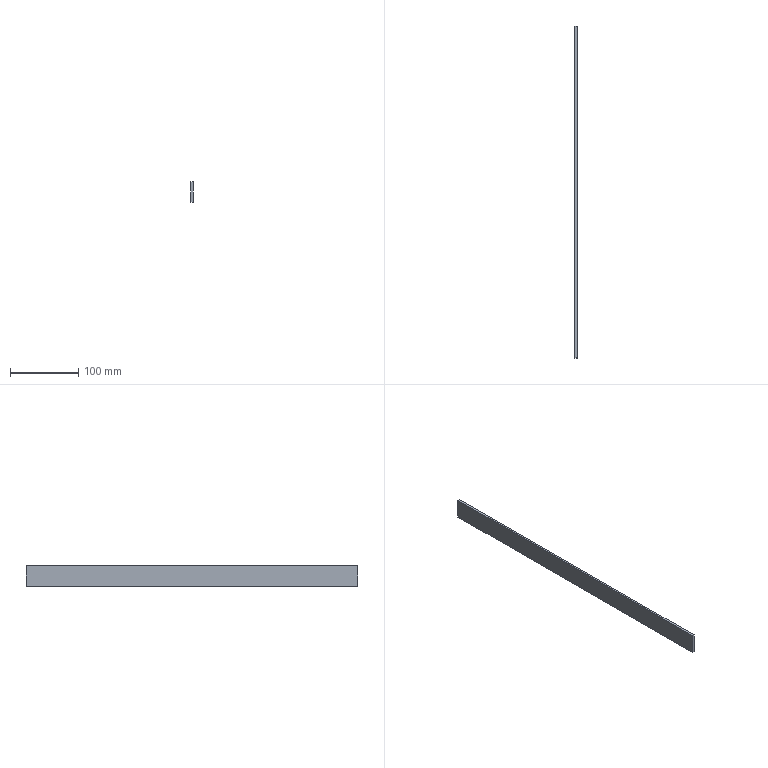Part | SolidWorks | 1 solid | 6 faces | box 3 x 485 x 30 mm | volume 43650 mm3 | plane 6
STEP:
#1=CARTESIAN_POINT('',(0.,242.5,15.));
#2=VERTEX_POINT('',#1);
#3=CARTESIAN_POINT('',(0.,-242.5,15.));
#4=VERTEX_POINT('',#3);
#5=CARTESIAN_POINT('',(0.,-242.5,15.));
#6=DIRECTION('',(0.,-1.,0.));
#7=VECTOR('',#6,1000.);
#8=LINE('',#5,#7);
#9=EDGE_CURVE('',#2,#4,#8,.T.);
#10=ORIENTED_EDGE('',*,*,#9,.F.);
#11=CARTESIAN_POINT('',(-3.,242.5,15.));
#12=VERTEX_POINT('',#11);
#13=CARTESIAN_POINT('',(-3.,242.5,15.));
#14=DIRECTION('',(1.,0.,0.));
#15=VECTOR('',#14,1000.);
#16=LINE('',#13,#15);
#17=EDGE_CURVE('',#12,#2,#16,.T.);
#18=ORIENTED_EDGE('',*,*,#17,.F.);
#19=CARTESIAN_POINT('',(-3.,-242.5,15.));
#20=VERTEX_POINT('',#19);
#21=CARTESIAN_POINT('',(-3.,-242.5,15.));
#22=DIRECTION('',(0.,-1.,0.));
#23=VECTOR('',#22,1000.);
#24=LINE('',#21,#23);
#25=EDGE_CURVE('',#12,#20,#24,.T.);
#26=ORIENTED_EDGE('',*,*,#25,.T.);
#27=CARTESIAN_POINT('',(-3.,-242.5,15.));
#28=DIRECTION('',(1.,0.,0.));
#29=VECTOR('',#28,1000.);
#30=LINE('',#27,#29);
#31=EDGE_CURVE('',#20,#4,#30,.T.);
#32=ORIENTED_EDGE('',*,*,#31,.T.);
#33=EDGE_LOOP('',(#10,#18,#26,#32));
#34=FACE_OUTER_BOUND('',#33,.T.);
#35=CARTESIAN_POINT('',(-3.,-242.5,15.));
#36=DIRECTION('',(0.,0.,1.));
#37=DIRECTION('',(1.,0.,0.));
#38=AXIS2_PLACEMENT_3D('',#35,#36,#37);
#39=PLANE('',#38);
#40=ADVANCED_FACE('',(#34),#39,.T.);
#41=CARTESIAN_POINT('',(0.,242.5,-15.));
#42=VERTEX_POINT('',#41);
#43=CARTESIAN_POINT('',(0.,242.5,-15.));
#44=DIRECTION('',(0.,0.,1.));
#45=VECTOR('',#44,1000.);
#46=LINE('',#43,#45);
#47=EDGE_CURVE('',#42,#2,#46,.T.);
#48=ORIENTED_EDGE('',*,*,#47,.F.);
#49=CARTESIAN_POINT('',(-3.,242.5,-15.));
#50=VERTEX_POINT('',#49);
#51=CARTESIAN_POINT('',(-3.,242.5,-15.));
#52=DIRECTION('',(1.,0.,0.));
#53=VECTOR('',#52,1000.);
#54=LINE('',#51,#53);
#55=EDGE_CURVE('',#50,#42,#54,.T.);
#56=ORIENTED_EDGE('',*,*,#55,.F.);
#57=CARTESIAN_POINT('',(-3.,242.5,-15.));
#58=DIRECTION('',(0.,0.,1.));
#59=VECTOR('',#58,1000.);
#60=LINE('',#57,#59);
#61=EDGE_CURVE('',#50,#12,#60,.T.);
#62=ORIENTED_EDGE('',*,*,#61,.T.);
#63=ORIENTED_EDGE('',*,*,#17,.T.);
#64=EDGE_LOOP('',(#48,#56,#62,#63));
#65=FACE_OUTER_BOUND('',#64,.T.);
#66=CARTESIAN_POINT('',(-3.,242.5,-15.));
#67=DIRECTION('',(0.,1.,0.));
#68=DIRECTION('',(0.,0.,1.));
#69=AXIS2_PLACEMENT_3D('',#66,#67,#68);
#70=PLANE('',#69);
#71=ADVANCED_FACE('',(#65),#70,.T.);
#72=CARTESIAN_POINT('',(0.,-242.5,-15.));
#73=VERTEX_POINT('',#72);
#74=CARTESIAN_POINT('',(0.,-242.5,-15.));
#75=DIRECTION('',(0.,1.,0.));
#76=VECTOR('',#75,1000.);
#77=LINE('',#74,#76);
#78=EDGE_CURVE('',#73,#42,#77,.T.);
#79=ORIENTED_EDGE('',*,*,#78,.F.);
#80=CARTESIAN_POINT('',(-3.,-242.5,-15.));
#81=VERTEX_POINT('',#80);
#82=CARTESIAN_POINT('',(-3.,-242.5,-15.));
#83=DIRECTION('',(1.,0.,0.));
#84=VECTOR('',#83,1000.);
#85=LINE('',#82,#84);
#86=EDGE_CURVE('',#81,#73,#85,.T.);
#87=ORIENTED_EDGE('',*,*,#86,.F.);
#88=CARTESIAN_POINT('',(-3.,-242.5,-15.));
#89=DIRECTION('',(0.,1.,0.));
#90=VECTOR('',#89,1000.);
#91=LINE('',#88,#90);
#92=EDGE_CURVE('',#81,#50,#91,.T.);
#93=ORIENTED_EDGE('',*,*,#92,.T.);
#94=ORIENTED_EDGE('',*,*,#55,.T.);
#95=EDGE_LOOP('',(#79,#87,#93,#94));
#96=FACE_OUTER_BOUND('',#95,.T.);
#97=CARTESIAN_POINT('',(-3.,-242.5,-15.));
#98=DIRECTION('',(0.,0.,-1.));
#99=DIRECTION('',(-1.,0.,0.));
#100=AXIS2_PLACEMENT_3D('',#97,#98,#99);
#101=PLANE('',#100);
#102=ADVANCED_FACE('',(#96),#101,.T.);
#103=CARTESIAN_POINT('',(0.,-242.5,-15.));
#104=DIRECTION('',(0.,0.,-1.));
#105=VECTOR('',#104,1000.);
#106=LINE('',#103,#105);
#107=EDGE_CURVE('',#4,#73,#106,.T.);
#108=ORIENTED_EDGE('',*,*,#107,.F.);
#109=ORIENTED_EDGE('',*,*,#31,.F.);
#110=CARTESIAN_POINT('',(-3.,-242.5,-15.));
#111=DIRECTION('',(0.,0.,-1.));
#112=VECTOR('',#111,1000.);
#113=LINE('',#110,#112);
#114=EDGE_CURVE('',#20,#81,#113,.T.);
#115=ORIENTED_EDGE('',*,*,#114,.T.);
#116=ORIENTED_EDGE('',*,*,#86,.T.);
#117=EDGE_LOOP('',(#108,#109,#115,#116));
#118=FACE_OUTER_BOUND('',#117,.T.);
#119=CARTESIAN_POINT('',(-3.,-242.5,-15.));
#120=DIRECTION('',(0.,-1.,0.));
#121=DIRECTION('',(0.,0.,-1.));
#122=AXIS2_PLACEMENT_3D('',#119,#120,#121);
#123=PLANE('',#122);
#124=ADVANCED_FACE('',(#118),#123,.T.);
#125=ORIENTED_EDGE('',*,*,#25,.F.);
#126=ORIENTED_EDGE('',*,*,#61,.F.);
#127=ORIENTED_EDGE('',*,*,#92,.F.);
#128=ORIENTED_EDGE('',*,*,#114,.F.);
#129=EDGE_LOOP('',(#125,#126,#127,#128));
#130=FACE_OUTER_BOUND('',#129,.T.);
#131=CARTESIAN_POINT('',(-3.,0.,0.));
#132=DIRECTION('',(1.,0.,0.));
#133=DIRECTION('',(0.,0.,-1.));
#134=AXIS2_PLACEMENT_3D('',#131,#132,#133);
#135=PLANE('',#134);
#136=ADVANCED_FACE('',(#130),#135,.F.);
#137=ORIENTED_EDGE('',*,*,#9,.T.);
#138=ORIENTED_EDGE('',*,*,#107,.T.);
#139=ORIENTED_EDGE('',*,*,#78,.T.);
#140=ORIENTED_EDGE('',*,*,#47,.T.);
#141=EDGE_LOOP('',(#137,#138,#139,#140));
#142=FACE_OUTER_BOUND('',#141,.T.);
#143=CARTESIAN_POINT('',(0.,0.,0.));
#144=DIRECTION('',(1.,0.,0.));
#145=DIRECTION('',(0.,0.,-1.));
#146=AXIS2_PLACEMENT_3D('',#143,#144,#145);
#147=PLANE('',#146);
#148=ADVANCED_FACE('',(#142),#147,.T.);
#149=CLOSED_SHELL('',(#40,#71,#102,#124,#136,#148));
#150=MANIFOLD_SOLID_BREP('',#149);
#151=CARTESIAN_POINT('',(0.,0.,0.));
#152=DIRECTION('',(0.,0.,1.));
#153=DIRECTION('',(1.,0.,0.));
#154=AXIS2_PLACEMENT_3D('',#151,#152,#153);
#155=(LENGTH_UNIT()NAMED_UNIT(*)SI_UNIT(.MILLI.,.METRE.));
#156=UNCERTAINTY_MEASURE_WITH_UNIT(LENGTH_MEASURE(0.00001),#155,'','');
#157=(NAMED_UNIT(*)PLANE_ANGLE_UNIT()SI_UNIT($,.RADIAN.));
#158=(NAMED_UNIT(*)SI_UNIT($,.STERADIAN.)SOLID_ANGLE_UNIT());
#159=(GEOMETRIC_REPRESENTATION_CONTEXT(3)GLOBAL_UNCERTAINTY_ASSIGNED_CONTEXT((#156))GLOBAL_UNIT_ASSIGNED_CONTEXT((#155,#157,#158))REPRESENTATION_CONTEXT('',''));
#160=ADVANCED_BREP_SHAPE_REPRESENTATION('',(#150,#154),#159);